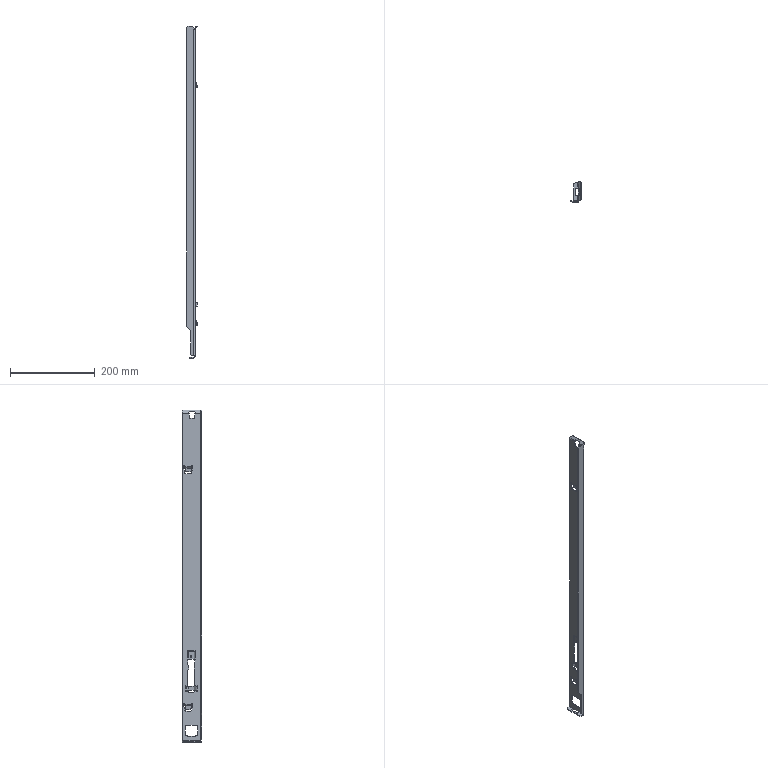Part | NX | features solid 2 | 1 solid | 233 faces | box 25.775 x 46.432 x 781.358 mm | volume 93860 mm3 | plane 133 | cylinder 94 | spline 6 | commonest cylinder face diameters 2 x22 1 x14 4 x11 1.86 x9 5.86 x9 0.5 x5